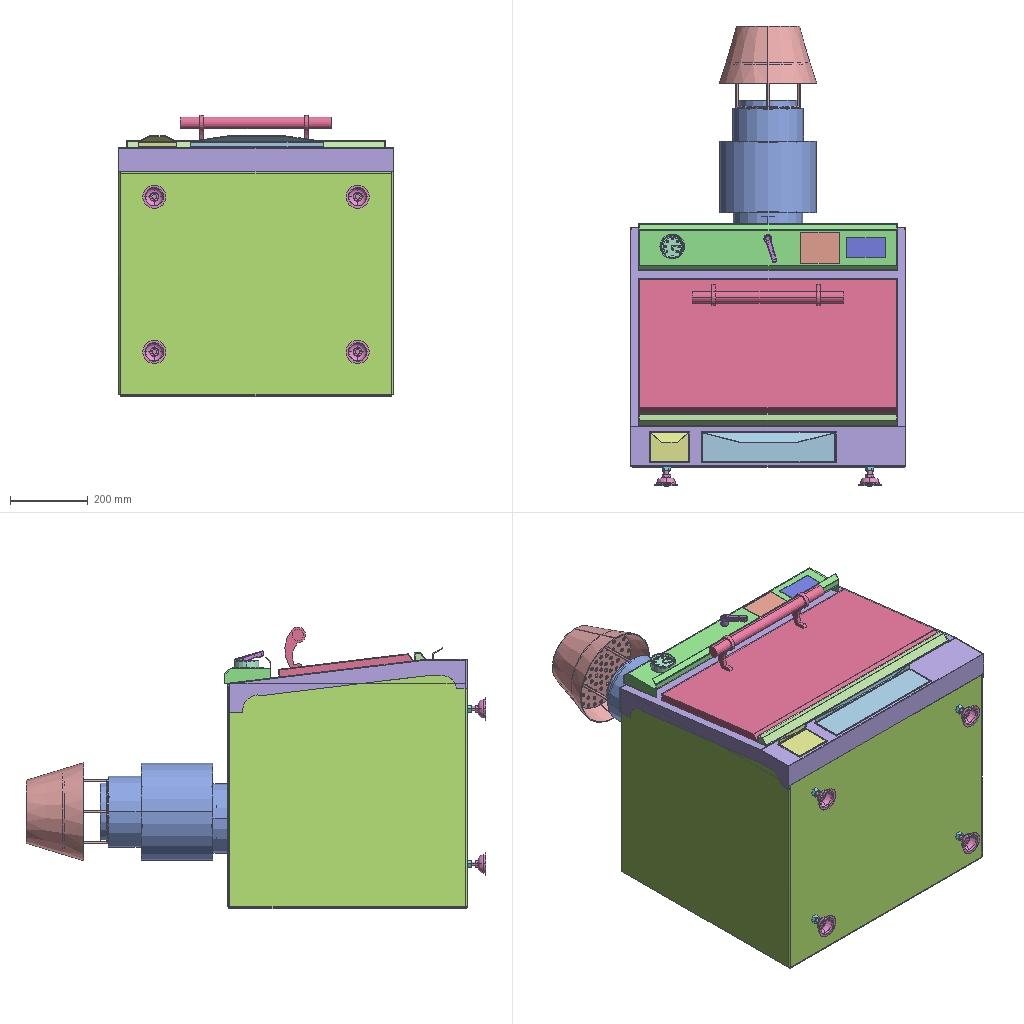Assembly | SolidWorks | 23 different items | 32 placed | box 710 x 1185 x 725 mm
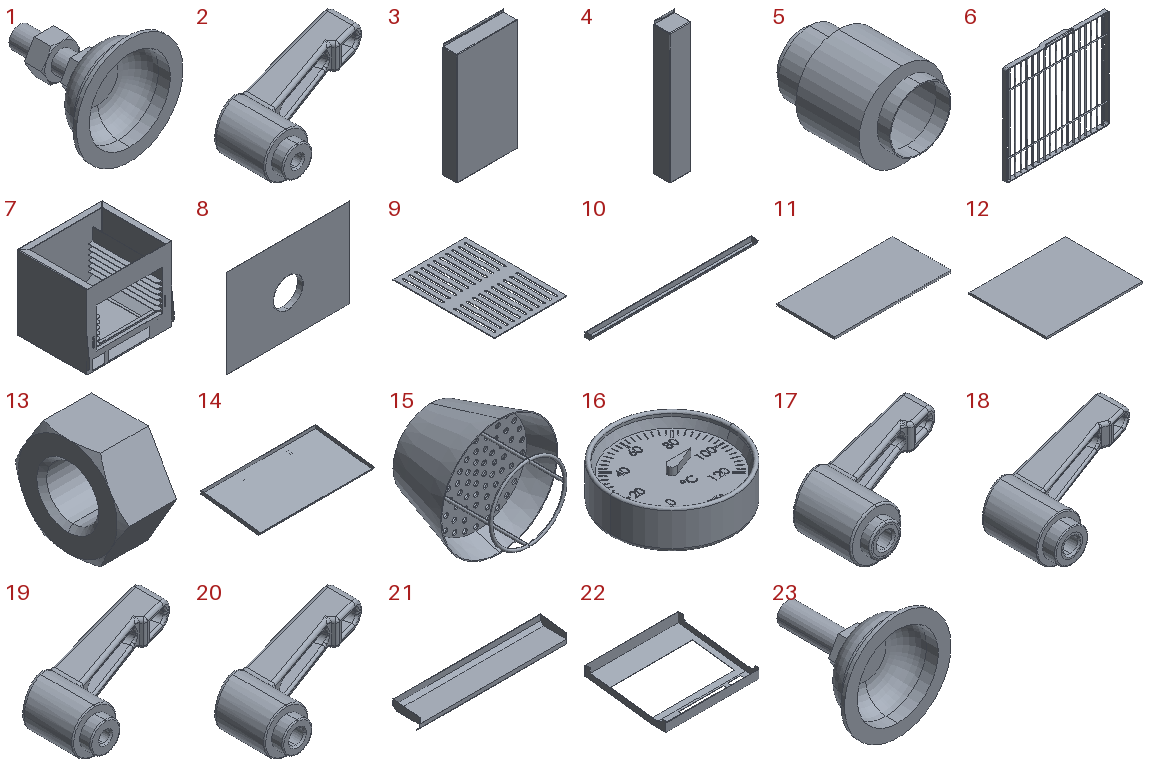Parts list (item | name | quantity | parent item | size | volume | features):
1 | (subassembly) | x4 | - | 60 x 62 x 60 mm | 16369 mm3 | -
2 | (subassembly) | x1 | - | 75 x 49.204 x 20.002 mm | 13893 mm3 | -
3 | - | x1 | - | 348 x 80 x 668.155 mm | 769690 mm3 | features EdgeFlange 3, FlatPattern 1, ICE 1, SMBaseFlange 1, SheetMetal 1
4 | - | x1 | - | 104 x 80 x 668.155 mm | 365737 mm3 | features EdgeFlange 3, FlatPattern 1, ICE 1, SMBaseFlange 1, SheetMetal 1
5 | - | x1 | - | 250 x 327 x 250 mm | 825128 mm3 | features ICE 1, Revolution 1, Shell 1
6 | - | x1 | - | 528 x 43 x 530 mm | 442043 mm3 | features ICE 3, LPattern 2, Sweep 2, Extrusion 1, Fillet 1, MirrorPattern 1
7 | - | x1 | - | 706 x 601.439 x 616 mm | 10499280 mm3 | features ICE 10, EdgeFlange 2, Fillet 2, Cut 1, FlatPattern 1, SMBaseFlange 1, SheetMetal 1
8 | - | x1 | - | 698 x 30 x 501 mm | 716095 mm3 | features ICE 2, FlatPattern 1, SMBaseFlange 1, SheetMetal 1
9 | - | x1 | - | 413 x 572 x 4 mm | 702671 mm3 | features Extrusion 1, ICE 1
10 | - | x1 | - | 665 x 29.785 x 21.93 mm | 75134 mm3 | features ICE 2, Extrusion 1
11 | - | x1 | - | 100 x 50 x 2 mm | 10000 mm3 | features Extrusion 1
12 | - | x1 | - | 100 x 80 x 2 mm | 16000 mm3 | features Extrusion 1
13 | - | x4 | in 1 | 10 x 21.939 x 19 mm | 2287 mm3 | features RefAxis 3, RevCut 2, 3DProfileFeature 1, ICE 1, Revolution 1
14 | - | x1 | - | 665 x 347.491 x 128.669 mm | 843762 mm3 | features ICE 5, Extrusion 1, LPattern 1
15 | - | x1 | - | 252.5 x 213 x 252.5 mm | 319111 mm3 | features ICE 3, Revolution 2, Shell 1, Sweep 1
16 | - | x1 | - | 64 x 64 x 20 mm | 43695 mm3 | features ICE 17, Fillet 3, CirPattern 1, Extrusion 1, MoveCopyBody 1, RevCut 1, Scale 1, Stock 1
17 | - | x1 | in 2 | 50 x 34.597 x 16.002 mm | 5701 mm3 | features BaseBody 1
18 | - | x1 | in 2 | 92.5 x 62.638 x 25.001 mm | 27128 mm3 | features BaseBody 1
19 | - | x1 | in 2 | 75 x 49.204 x 20.002 mm | 13893 mm3 | features BaseBody 1
20 | - | x1 | in 2 | 75 x 49.204 x 20.002 mm | 13686 mm3 | features BaseBody 1
21 | - | x1 | - | 665 x 120 x 68.021 mm | 255625 mm3 | features ICE 2, Chamfer 1, Extrusion 1, Shell 1
22 | - | x1 | - | 710 x 618 x 137 mm | 789062 mm3 | features ICE 5, Cut 1, Extrusion 1
23 | - | x4 | in 1 | 60 x 62 x 60 mm | 14083 mm3 | features RefAxis 6, 3DProfileFeature 2, Revolution 2, Cut 1, ICE 1, RevCut 1
Mates (type | each side: item.copy, entity, surface, feature):
In the top assembly
Coincident | 15.1 plane | assembly plane | 3 times
Concentric | 15.1 face cone Revolve1 | 5.1 face cylinder Revolve1
DistanceDim | 15.1 plane | 5.1 face plane Revolve1
Coincident | 15.1 plane | 5.1 plane
Coincident | 5.1 plane | 7.1 plane
Parallel | 5.1 face plane Revolve1 | 7.1 face plane Base-Flange1
DistanceDim | 5.1 plane | 7.1 face plane Edge-Flange1
Coincident | 7.1 plane | 8.1 plane
Coincident | 7.1 face plane Edge-Flange2 | 8.1 face plane Base-Flange1
Coincident | 7.1 face plane Boss-Extrude8 | 9.1 face plane Boss-Extrude1
Coincident | 7.1 plane | 9.1 plane
Coincident | 7.1 face plane Edge-Flange1 | 9.1 face plane Boss-Extrude1
Coincident | 7.1 face plane Boss-Extrude7 | 6.1 face plane Boss-Extrude1
Coincident | 7.1 plane | 6.1 plane
DistanceDim | 8.1 face plane Base-Flange1 | 7.1 face plane Edge-Flange1
Coincident | 5.1 face plane Boss-Extrude1 | 8.1 face plane Base-Flange1
Coincident | 7.1 face plane Edge-Flange1 | 22.1 face plane Boss-Extrude1
Coincident | 7.1 face plane Edge-Flange2 | 22.1 face plane Boss-Extrude2
DistanceDim | 22.1 face plane Boss-Extrude1 | 7.1 face plane Edge-Flange1
Coincident | 22.1 face plane Boss-Extrude1 | 21.1 face plane Boss-Extrude1
Coincident | 7.1 plane | 21.1 plane
DistanceDim | 21.1 face plane Boss-Extrude1 | 22.1 face plane Boss-Extrude1
Coincident | 22.1 face plane Boss-Extrude1 | 14.1 face plane Boss-Extrude1
Parallel | 22.1 face plane Boss-Extrude1 | 14.1 face plane Boss-Extrude1
Width | 14.1 face plane Boss-Extrude1 | 14.1 face plane Boss-Extrude3 | 22.1 face plane Boss-Extrude3 | 22.1 face plane Boss-Extrude1
DistanceDim | 14.1 face plane Boss-Extrude1 | 21.1 face plane Boss-Extrude1
Coincident | 22.1 face plane Cut-Extrude3 | 3.1 face plane Base-Flange1
Coincident | 22.1 face plane Cut-Extrude3 | 3.1 face plane Edge-Flange1
Coincident | 22.1 face plane Boss-Extrude1 | 3.1 face plane Edge-Flange1
Coincident | 22.1 face plane Cut-Extrude3 | 4.1 face plane Base-Flange1
Coincident | 22.1 face plane Cut-Extrude3 | 4.1 face plane Edge-Flange1
Coincident | 3.1 face plane Edge-Flange1 | 4.1 face plane Edge-Flange1
Coincident | 21.1 face plane Boss-Extrude1 | 20.1 face
Coincident | 21.1 face plane Boss-Extrude1 | 16.1 face plane Boss-Extrude1
Coincident | 21.1 face plane Boss-Extrude1 | 12.1 face plane Boss-Extrude1
Parallel | 21.1 face plane Boss-Extrude1 | 12.1 face plane Boss-Extrude1
Coincident | 21.1 face plane Boss-Extrude1 | 11.1 face plane Boss-Extrude1
Parallel | 21.1 face plane Boss-Extrude1 | 11.1 face plane Boss-Extrude1
Coincident | 7.1 face plane Base-Flange1 | 13.1 face plane Revolve1
Coincident | 22.1 face plane Boss-Extrude1 | 10.1 face plane Boss-Extrude1
Coincident | 14.1 face plane Boss-Extrude1 | 10.1 face plane Boss-Extrude1
In subassembly 1
Coincident | 23.1 axis | 13.2 axis | 3 times
PlanarAngleDim | 13.2 plane | 23.1 plane